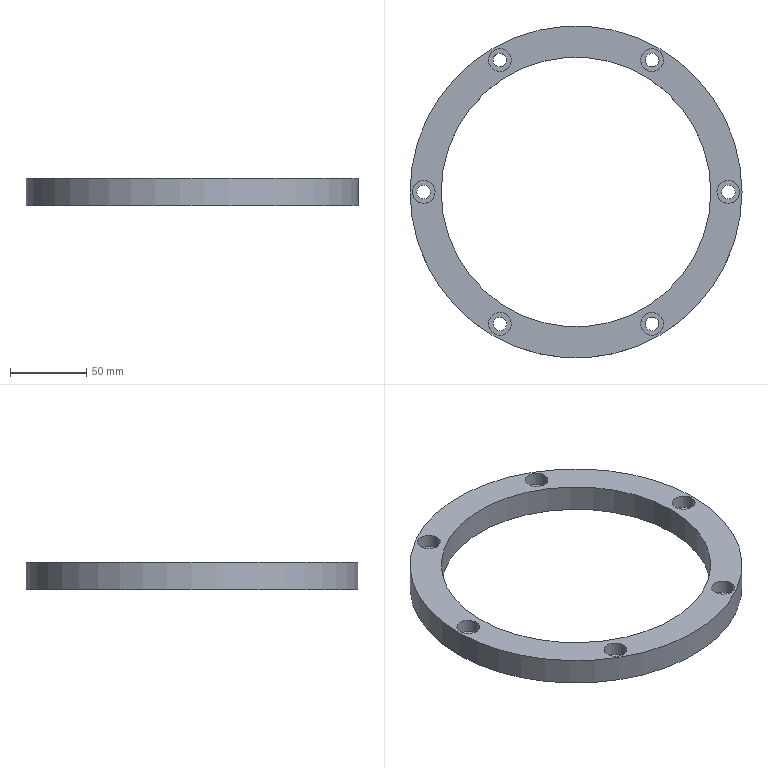NC program | NX | posted with a generic post | part box 218 x 218 x 18 mm
Whole program:
N10 G17 G21 G94 G90
(DRILLING , TOOL : ZXZ)
N12 T01 M6
N14 G54
N16 G17 G0 G90 X100. Y0. S3000 M3
N18 G43 Z30. H1
N20 G94 G81 G98 Z-1. F200. R3.
N22 X50. Y86.603
N24 X-50.
N26 X-100. Y0.
N28 X-50. Y-86.603
N30 X50.
N32 G80
N34 G0 X50. Y-86.603 Z30.
N36 M5
(DRILLING_COPY , TOOL : 9.0ZT)
N38 T09 M6
N40 G54
N42 G17 G0 G90 X100. Y0. S1203 M3
N44 G43 Z30. H9
N46 G94 G83 G98 Z-22.204 F150. Q2. R3.
N48 X50. Y86.603
N50 X-50.
N52 X-100. Y0.
N54 X-50. Y-86.603
N56 X50.
N58 G80
N60 G0 X50. Y-86.603 Z30.
N62 M5
(ZLEVEL_PROFILE_1_COPY_1 , TOOL : D6A45)
N64 T07 M6
N66 G54
N68 G17 G0 G90 X-48.895 Y91.913 S6500 M3
N70 G43 Z30. H7
N72 Z0.
N74 G94 G1 Z-1. F1000.
N76 X-49.48 Y92.927
N78 G3 X-50. Y93.227 R0.6
N80 X-56.624 Y86.603 R6.624
N82 X-50. Y93.227 R-6.624
N84 X-50.52 Y92.927 R0.6
N86 G1 X-51.105 Y91.913
N88 Z0.
N90 G0 Z30.
N92 X51.105
N94 Z0.
N96 G1 Z-1.
N98 X50.52 Y92.927
N100 G3 X50. Y93.227 R0.6
N102 X43.376 Y86.603 R6.624
N104 X50. Y93.227 R-6.624
N106 X49.48 Y92.927 R0.6
N108 G1 X48.895 Y91.913
N110 Z0.
N112 G0 Z30.
N114 X105.311 Y-1.105
N116 Z0.
N118 G1 Z-1.
N120 X106.324 Y-0.52
N122 G3 X106.624 Y0. R0.6
N124 X100. Y6.624 R6.624
N126 X106.624 Y0. R-6.624
N128 X106.324 Y0.52 R0.6
N130 G1 X105.311 Y1.105
N132 Z0.
N134 G0 Z30.
N136 X-105.311
N138 Z0.
N140 G1 Z-1.
N142 X-106.324 Y0.52
N144 G3 X-106.624 Y0. R0.6
N146 X-100. Y-6.624 R6.624
N148 X-106.624 Y0. R-6.624
N150 X-106.324 Y-0.52 R0.6
N152 G1 X-105.311 Y-1.105
N154 Z0.
N156 G0 Z30.
N158 X-51.105 Y-91.913
N160 Z0.
N162 G1 Z-1.
N164 X-50.52 Y-92.927
N166 G3 X-50. Y-93.227 R0.6
N168 X-43.376 Y-86.603 R6.624
N170 X-50. Y-93.227 R-6.624
N172 X-49.48 Y-92.927 R0.6
N174 G1 X-48.895 Y-91.913
N176 Z0.
N178 G0 Z30.
N180 X48.895
N182 Z0.
N184 G1 Z-1.
N186 X49.48 Y-92.927
N188 G3 X50. Y-93.227 R0.6
N190 X56.624 Y-86.603 R6.624
N192 X50. Y-93.227 R-6.624
N194 X50.52 Y-92.927 R0.6
N196 G1 X51.105 Y-91.913
N198 Z0.
N200 G0 Z30.
N202 M5
N204 M2